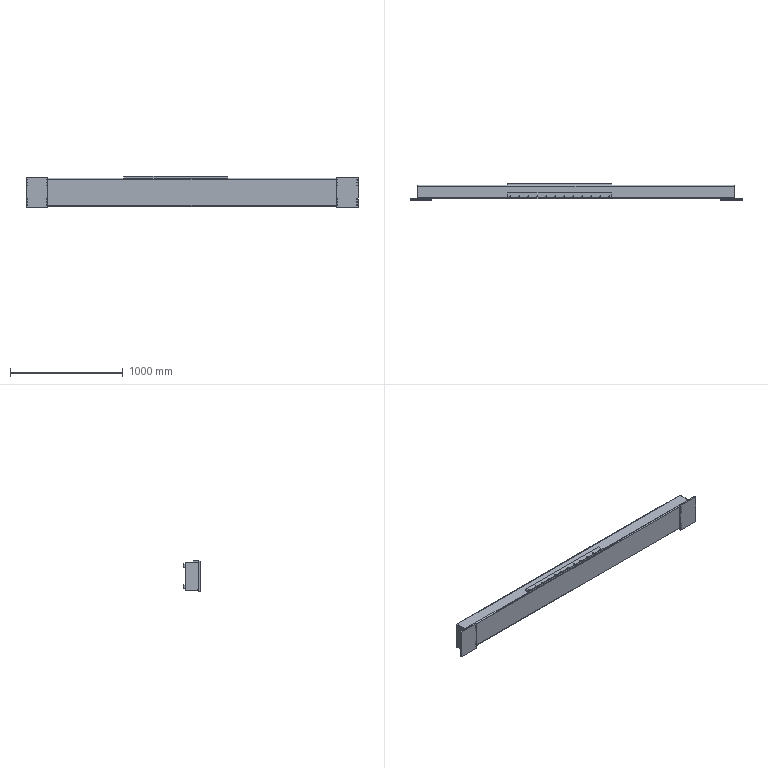Part | SolidWorks | features HoleWzd 7, ICE 5, MirrorSolid 3, Chamfer 2, WeldMemberFeat 1, WeldmentFeature 1 | 10 solids | 304 faces | box 2945 x 142 x 275 mm | volume 8968186 mm3 | cylinder 222 | plane 82 | commonest cylinder face diameters 6.8 x88 6.6 x72 11 x24 14 x20 5 x14 20 x4